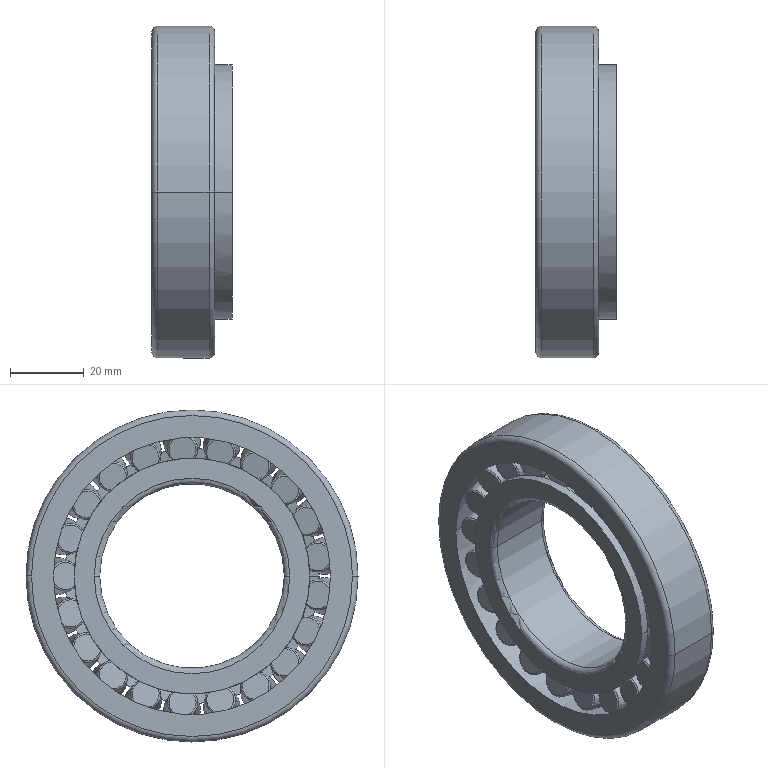Part | SolidWorks | features Revolution 3, CirPattern 1 | 1 solid | 196 faces | box 21.75 x 90 x 90 mm | volume 63957 mm3 | torus 92 | cone 50 | plane 46 | cylinder 8 | commonest cylinder face diameters 50 x2 63.859 x2 69.068 x2 90 x2